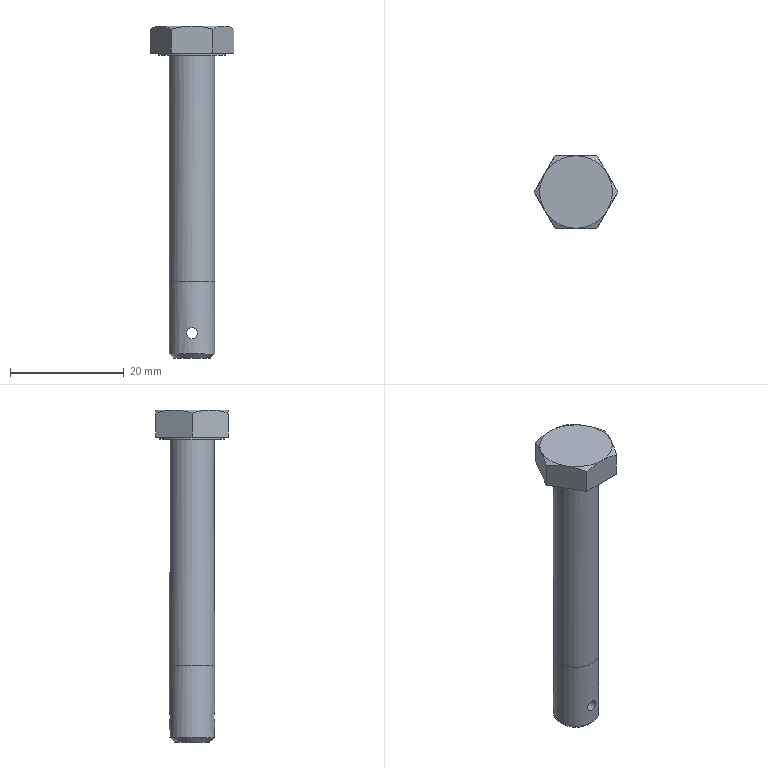Part | NX | features solid 2 | 1 solid | 21 faces | box 14.723 x 12.751 x 58.363 mm | volume 3315 mm3 | plane 10 | cone 7 | cylinder 4 | commonest cylinder face diameters 7.938 x2 1.93 x1 11.684 x1
STEP:
#1=CARTESIAN_POINT('',(0.,-3.969,-54.962));
#2=VERTEX_POINT('',#1);
#3=CARTESIAN_POINT('',(0.7571,-3.91,-54.753));
#4=CARTESIAN_POINT('',(-0.000144,-3.998,-55.067));
#5=CARTESIAN_POINT('',(-0.7565,-3.91,-54.753));
#6=CARTESIAN_POINT('',(-1.07,-3.819,-53.998));
#7=CARTESIAN_POINT('',(-0.7564,-3.91,-53.241));
#8=CARTESIAN_POINT('',(-0.0004429,-3.998,-52.928));
#9=CARTESIAN_POINT('',(0.7557,-3.91,-53.24));
#10=CARTESIAN_POINT('',(1.07,-3.819,-53.997));
#11=CARTESIAN_POINT('',(0.7571,-3.91,-54.753));
#12=CARTESIAN_POINT('',(-0.000144,-3.998,-55.067));
#13=CARTESIAN_POINT('',(-0.7565,-3.91,-54.753));
#14=B_SPLINE_CURVE_WITH_KNOTS('',3,(#3,#4,#5,#6,#7,#8,#9,#10,#11,#12,#13),.UNSPECIFIED.,.T.,.F.,(1,1,1,1,1,1,1,1,1,1,1,1,1,1,1),(-0.002271,-0.001514,-0.0007572,0.,0.0007572,0.001514,0.002271,0.003029,0.003786,0.004543,0.0053,0.006057,0.006814,0.007572,0.008329),.UNSPECIFIED.);
#15=EDGE_CURVE('',#2,#2,#14,.T.);
#16=ORIENTED_EDGE('',*,*,#15,.T.);
#17=EDGE_LOOP('',(#16));
#18=FACE_BOUND('',#17,.T.);
#19=CARTESIAN_POINT('',(-3.969,0.,-44.869));
#20=VERTEX_POINT('',#19);
#21=CARTESIAN_POINT('',(-3.11,3.11,-44.869));
#22=CARTESIAN_POINT('',(-4.398,0.,-44.869));
#23=CARTESIAN_POINT('',(-3.11,-3.11,-44.869));
#24=CARTESIAN_POINT('',(0.,-4.398,-44.869));
#25=CARTESIAN_POINT('',(3.11,-3.11,-44.869));
#26=CARTESIAN_POINT('',(4.398,0.,-44.869));
#27=CARTESIAN_POINT('',(3.11,3.11,-44.869));
#28=CARTESIAN_POINT('',(0.,4.398,-44.869));
#29=CARTESIAN_POINT('',(-3.11,3.11,-44.869));
#30=CARTESIAN_POINT('',(-4.398,0.,-44.869));
#31=CARTESIAN_POINT('',(-3.11,-3.11,-44.869));
#32=B_SPLINE_CURVE_WITH_KNOTS('',3,(#21,#22,#23,#24,#25,#26,#27,#28,#29,#30,#31),.UNSPECIFIED.,.T.,.F.,(1,1,1,1,1,1,1,1,1,1,1,1,1,1,1),(-0.375,-0.25,-0.125,0.,0.125,0.25,0.375,0.5,0.625,0.75,0.875,1.,1.125,1.25,1.375),.UNSPECIFIED.);
#33=EDGE_CURVE('',#20,#20,#32,.T.);
#34=ORIENTED_EDGE('',*,*,#33,.F.);
#35=EDGE_LOOP('',(#34));
#36=FACE_BOUND('',#35,.T.);
#37=CARTESIAN_POINT('',(-3.969,0.,-57.575));
#38=VERTEX_POINT('',#37);
#39=CARTESIAN_POINT('',(0.,0.,-57.575));
#40=DIRECTION('',(0.,0.,-1.));
#41=DIRECTION('',(-1.,0.,0.));
#42=AXIS2_PLACEMENT_3D('',#39,#40,#41);
#43=CIRCLE('',#42,3.969);
#44=EDGE_CURVE('',#38,#38,#43,.T.);
#45=ORIENTED_EDGE('',*,*,#44,.F.);
#46=EDGE_LOOP('',(#45));
#47=FACE_BOUND('',#46,.T.);
#48=CARTESIAN_POINT('',(0.,3.969,-54.962));
#49=VERTEX_POINT('',#48);
#50=CARTESIAN_POINT('',(-0.7571,3.91,-54.753));
#51=CARTESIAN_POINT('',(0.000144,3.998,-55.067));
#52=CARTESIAN_POINT('',(0.7565,3.91,-54.753));
#53=CARTESIAN_POINT('',(1.07,3.819,-53.998));
#54=CARTESIAN_POINT('',(0.7564,3.91,-53.241));
#55=CARTESIAN_POINT('',(0.0004429,3.998,-52.928));
#56=CARTESIAN_POINT('',(-0.7557,3.91,-53.24));
#57=CARTESIAN_POINT('',(-1.07,3.819,-53.997));
#58=CARTESIAN_POINT('',(-0.7571,3.91,-54.753));
#59=CARTESIAN_POINT('',(0.000144,3.998,-55.067));
#60=CARTESIAN_POINT('',(0.7565,3.91,-54.753));
#61=B_SPLINE_CURVE_WITH_KNOTS('',3,(#50,#51,#52,#53,#54,#55,#56,#57,#58,#59,#60),.UNSPECIFIED.,.T.,.F.,(1,1,1,1,1,1,1,1,1,1,1,1,1,1,1),(-0.002271,-0.001514,-0.0007572,0.,0.0007572,0.001514,0.002271,0.003029,0.003786,0.004543,0.0053,0.006057,0.006814,0.007572,0.008329),.UNSPECIFIED.);
#62=EDGE_CURVE('',#49,#49,#61,.T.);
#63=ORIENTED_EDGE('',*,*,#62,.T.);
#64=EDGE_LOOP('',(#63));
#65=FACE_BOUND('',#64,.T.);
#66=CARTESIAN_POINT('',(0.,0.,0.));
#67=DIRECTION('',(0.,0.,-1.));
#68=DIRECTION('',(-1.,0.,0.));
#69=AXIS2_PLACEMENT_3D('',#66,#67,#68);
#70=CYLINDRICAL_SURFACE('',#69,3.969);
#71=ADVANCED_FACE('',(#18,#36,#47,#65),#70,.T.);
#72=CARTESIAN_POINT('',(-3.969,0.,-5.182));
#73=VERTEX_POINT('',#72);
#74=CARTESIAN_POINT('',(0.,0.,-5.182));
#75=DIRECTION('',(0.,0.,-1.));
#76=DIRECTION('',(-1.,0.,0.));
#77=AXIS2_PLACEMENT_3D('',#74,#75,#76);
#78=CIRCLE('',#77,3.969);
#79=EDGE_CURVE('',#73,#73,#78,.T.);
#80=ORIENTED_EDGE('',*,*,#79,.T.);
#81=EDGE_LOOP('',(#80));
#82=FACE_BOUND('',#81,.T.);
#83=ORIENTED_EDGE('',*,*,#33,.T.);
#84=EDGE_LOOP('',(#83));
#85=FACE_BOUND('',#84,.T.);
#86=CARTESIAN_POINT('',(0.,0.,0.));
#87=DIRECTION('',(0.,0.,-1.));
#88=DIRECTION('',(-1.,0.,0.));
#89=AXIS2_PLACEMENT_3D('',#86,#87,#88);
#90=CYLINDRICAL_SURFACE('',#89,3.969);
#91=ADVANCED_FACE('',(#82,#85),#90,.T.);
#92=CARTESIAN_POINT('',(-7.362,0.,-4.775));
#93=VERTEX_POINT('',#92);
#94=CARTESIAN_POINT('',(-3.681,6.375,-4.775));
#95=VERTEX_POINT('',#94);
#96=CARTESIAN_POINT('',(-4.061,5.717,-4.775));
#97=DIRECTION('',(0.5,0.866,0.));
#98=VECTOR('',#97,1000.);
#99=LINE('',#96,#98);
#100=EDGE_CURVE('',#93,#95,#99,.T.);
#101=ORIENTED_EDGE('',*,*,#100,.T.);
#102=CARTESIAN_POINT('',(3.681,6.375,-4.775));
#103=VERTEX_POINT('',#102);
#104=CARTESIAN_POINT('',(5.842,6.375,-4.775));
#105=DIRECTION('',(1.,0.,0.));
#106=VECTOR('',#105,1000.);
#107=LINE('',#104,#106);
#108=EDGE_CURVE('',#95,#103,#107,.T.);
#109=ORIENTED_EDGE('',*,*,#108,.T.);
#110=CARTESIAN_POINT('',(7.362,0.,-4.775));
#111=VERTEX_POINT('',#110);
#112=CARTESIAN_POINT('',(6.982,0.658,-4.775));
#113=DIRECTION('',(0.5,-0.866,0.));
#114=VECTOR('',#113,1000.);
#115=LINE('',#112,#114);
#116=EDGE_CURVE('',#103,#111,#115,.T.);
#117=ORIENTED_EDGE('',*,*,#116,.T.);
#118=CARTESIAN_POINT('',(3.681,-6.375,-4.775));
#119=VERTEX_POINT('',#118);
#120=CARTESIAN_POINT('',(6.982,-0.658,-4.775));
#121=DIRECTION('',(-0.5,-0.866,0.));
#122=VECTOR('',#121,1000.);
#123=LINE('',#120,#122);
#124=EDGE_CURVE('',#111,#119,#123,.T.);
#125=ORIENTED_EDGE('',*,*,#124,.T.);
#126=CARTESIAN_POINT('',(-3.681,-6.375,-4.775));
#127=VERTEX_POINT('',#126);
#128=CARTESIAN_POINT('',(5.842,-6.375,-4.775));
#129=DIRECTION('',(-1.,0.,0.));
#130=VECTOR('',#129,1000.);
#131=LINE('',#128,#130);
#132=EDGE_CURVE('',#119,#127,#131,.T.);
#133=ORIENTED_EDGE('',*,*,#132,.T.);
#134=CARTESIAN_POINT('',(-4.061,-5.717,-4.775));
#135=DIRECTION('',(-0.5,0.866,0.));
#136=VECTOR('',#135,1000.);
#137=LINE('',#134,#136);
#138=EDGE_CURVE('',#127,#93,#137,.T.);
#139=ORIENTED_EDGE('',*,*,#138,.T.);
#140=EDGE_LOOP('',(#101,#109,#117,#125,#133,#139));
#141=FACE_BOUND('',#140,.T.);
#142=CARTESIAN_POINT('',(-5.842,0.,-4.775));
#143=VERTEX_POINT('',#142);
#144=CARTESIAN_POINT('',(0.,0.,-4.775));
#145=DIRECTION('',(0.,0.,-1.));
#146=DIRECTION('',(-1.,0.,0.));
#147=AXIS2_PLACEMENT_3D('',#144,#145,#146);
#148=CIRCLE('',#147,5.842);
#149=EDGE_CURVE('',#143,#143,#148,.T.);
#150=ORIENTED_EDGE('',*,*,#149,.F.);
#151=EDGE_LOOP('',(#150));
#152=FACE_BOUND('',#151,.T.);
#153=CARTESIAN_POINT('',(5.842,0.,-4.775));
#154=DIRECTION('',(0.,0.,-1.));
#155=DIRECTION('',(-1.,0.,0.));
#156=AXIS2_PLACEMENT_3D('',#153,#154,#155);
#157=PLANE('',#156);
#158=ADVANCED_FACE('',(#141,#152),#157,.T.);
#159=CARTESIAN_POINT('',(-3.181,0.,-58.363));
#160=VERTEX_POINT('',#159);
#161=CARTESIAN_POINT('',(0.,0.,-58.363));
#162=DIRECTION('',(0.,0.,-1.));
#163=DIRECTION('',(-1.,0.,0.));
#164=AXIS2_PLACEMENT_3D('',#161,#162,#163);
#165=CIRCLE('',#164,3.181);
#166=EDGE_CURVE('',#160,#160,#165,.T.);
#167=ORIENTED_EDGE('',*,*,#166,.T.);
#168=EDGE_LOOP('',(#167));
#169=FACE_BOUND('',#168,.T.);
#170=CARTESIAN_POINT('',(0.,0.,-58.363));
#171=DIRECTION('',(0.,0.,-1.));
#172=DIRECTION('',(-1.,0.,0.));
#173=AXIS2_PLACEMENT_3D('',#170,#171,#172);
#174=PLANE('',#173);
#175=ADVANCED_FACE('',(#169),#174,.T.);
#176=ORIENTED_EDGE('',*,*,#44,.T.);
#177=EDGE_LOOP('',(#176));
#178=FACE_BOUND('',#177,.T.);
#179=ORIENTED_EDGE('',*,*,#166,.F.);
#180=EDGE_LOOP('',(#179));
#181=FACE_BOUND('',#180,.T.);
#182=CARTESIAN_POINT('',(0.,0.,-58.363));
#183=DIRECTION('',(0.,0.,1.));
#184=DIRECTION('',(1.,0.,0.));
#185=AXIS2_PLACEMENT_3D('',#182,#183,#184);
#186=CONICAL_SURFACE('',#185,3.181,0.7854);
#187=ADVANCED_FACE('',(#178,#181),#186,.T.);
#188=CARTESIAN_POINT('',(-5.842,0.,-5.182));
#189=VERTEX_POINT('',#188);
#190=CARTESIAN_POINT('',(0.,0.,-5.182));
#191=DIRECTION('',(0.,0.,-1.));
#192=DIRECTION('',(-1.,0.,0.));
#193=AXIS2_PLACEMENT_3D('',#190,#191,#192);
#194=CIRCLE('',#193,5.842);
#195=EDGE_CURVE('',#189,#189,#194,.T.);
#196=ORIENTED_EDGE('',*,*,#195,.T.);
#197=EDGE_LOOP('',(#196));
#198=FACE_BOUND('',#197,.T.);
#199=ORIENTED_EDGE('',*,*,#79,.F.);
#200=EDGE_LOOP('',(#199));
#201=FACE_BOUND('',#200,.T.);
#202=CARTESIAN_POINT('',(3.969,0.,-5.182));
#203=DIRECTION('',(0.,0.,-1.));
#204=DIRECTION('',(-1.,0.,0.));
#205=AXIS2_PLACEMENT_3D('',#202,#203,#204);
#206=PLANE('',#205);
#207=ADVANCED_FACE('',(#198,#201),#206,.T.);
#208=ORIENTED_EDGE('',*,*,#149,.T.);
#209=EDGE_LOOP('',(#208));
#210=FACE_BOUND('',#209,.T.);
#211=ORIENTED_EDGE('',*,*,#195,.F.);
#212=EDGE_LOOP('',(#211));
#213=FACE_BOUND('',#212,.T.);
#214=CARTESIAN_POINT('',(0.,0.,0.));
#215=DIRECTION('',(0.,0.,-1.));
#216=DIRECTION('',(-1.,0.,0.));
#217=AXIS2_PLACEMENT_3D('',#214,#215,#216);
#218=CYLINDRICAL_SURFACE('',#217,5.842);
#219=ADVANCED_FACE('',(#210,#213),#218,.T.);
#220=ORIENTED_EDGE('',*,*,#108,.F.);
#221=CARTESIAN_POINT('',(-3.681,6.375,-0.5694));
#222=VERTEX_POINT('',#221);
#223=CARTESIAN_POINT('',(-3.681,6.375,-64.199));
#224=DIRECTION('',(0.,0.,1.));
#225=VECTOR('',#224,1000.);
#226=LINE('',#223,#225);
#227=EDGE_CURVE('',#95,#222,#226,.T.);
#228=ORIENTED_EDGE('',*,*,#227,.T.);
#229=CARTESIAN_POINT('',(0.,6.375,0.));
#230=VERTEX_POINT('',#229);
#231=CARTESIAN_POINT('',(-3.681,6.375,-0.5694));
#232=CARTESIAN_POINT('',(-2.484,6.375,-0.2238));
#233=CARTESIAN_POINT('',(-1.244,6.375,0.));
#234=CARTESIAN_POINT('',(0.,6.375,0.));
#235=B_SPLINE_CURVE_WITH_KNOTS('',3,(#231,#232,#233,#234),.UNSPECIFIED.,.F.,.F.,(4,4),(0.006567,0.01029),.UNSPECIFIED.);
#236=EDGE_CURVE('',#230,#222,#235,.F.);
#237=ORIENTED_EDGE('',*,*,#236,.F.);
#238=CARTESIAN_POINT('',(3.681,6.375,-0.5694));
#239=VERTEX_POINT('',#238);
#240=CARTESIAN_POINT('',(0.,6.375,0.));
#241=CARTESIAN_POINT('',(1.245,6.375,0.));
#242=CARTESIAN_POINT('',(2.49,6.375,-0.2258));
#243=CARTESIAN_POINT('',(3.681,6.375,-0.5694));
#244=B_SPLINE_CURVE_WITH_KNOTS('',3,(#240,#241,#242,#243),.UNSPECIFIED.,.F.,.F.,(4,4),(0.01029,0.01402),.UNSPECIFIED.);
#245=EDGE_CURVE('',#239,#230,#244,.F.);
#246=ORIENTED_EDGE('',*,*,#245,.F.);
#247=CARTESIAN_POINT('',(3.681,6.375,-64.199));
#248=DIRECTION('',(0.,0.,1.));
#249=VECTOR('',#248,1000.);
#250=LINE('',#247,#249);
#251=EDGE_CURVE('',#103,#239,#250,.T.);
#252=ORIENTED_EDGE('',*,*,#251,.F.);
#253=EDGE_LOOP('',(#220,#228,#237,#246,#252));
#254=FACE_BOUND('',#253,.T.);
#255=CARTESIAN_POINT('',(3.681,6.375,-64.199));
#256=DIRECTION('',(0.,1.,0.));
#257=DIRECTION('',(0.,0.,1.));
#258=AXIS2_PLACEMENT_3D('',#255,#256,#257);
#259=PLANE('',#258);
#260=ADVANCED_FACE('',(#254),#259,.T.);
#261=ORIENTED_EDGE('',*,*,#100,.F.);
#262=CARTESIAN_POINT('',(-7.362,0.,-0.5694));
#263=VERTEX_POINT('',#262);
#264=CARTESIAN_POINT('',(-7.362,0.,-64.199));
#265=DIRECTION('',(0.,0.,1.));
#266=VECTOR('',#265,1000.);
#267=LINE('',#264,#266);
#268=EDGE_CURVE('',#93,#263,#267,.T.);
#269=ORIENTED_EDGE('',*,*,#268,.T.);
#270=CARTESIAN_POINT('',(-5.521,3.188,0.));
#271=VERTEX_POINT('',#270);
#272=CARTESIAN_POINT('',(-5.521,3.188,0.));
#273=CARTESIAN_POINT('',(-6.146,2.106,0.));
#274=CARTESIAN_POINT('',(-6.761,1.04,-0.2227));
#275=CARTESIAN_POINT('',(-7.362,0.,-0.5694));
#276=B_SPLINE_CURVE_WITH_KNOTS('',3,(#272,#273,#274,#275),.UNSPECIFIED.,.F.,.F.,(4,4),(0.003725,0.007435),.UNSPECIFIED.);
#277=EDGE_CURVE('',#271,#263,#276,.T.);
#278=ORIENTED_EDGE('',*,*,#277,.F.);
#279=CARTESIAN_POINT('',(-3.681,6.375,-0.5694));
#280=CARTESIAN_POINT('',(-4.283,5.332,-0.2218));
#281=CARTESIAN_POINT('',(-4.894,4.274,0.));
#282=CARTESIAN_POINT('',(-5.521,3.188,0.));
#283=B_SPLINE_CURVE_WITH_KNOTS('',3,(#279,#280,#281,#282),.UNSPECIFIED.,.F.,.F.,(4,4),(0.000000238,0.003725),.UNSPECIFIED.);
#284=EDGE_CURVE('',#222,#271,#283,.T.);
#285=ORIENTED_EDGE('',*,*,#284,.F.);
#286=ORIENTED_EDGE('',*,*,#227,.F.);
#287=EDGE_LOOP('',(#261,#269,#278,#285,#286));
#288=FACE_BOUND('',#287,.T.);
#289=CARTESIAN_POINT('',(-3.681,6.375,-64.199));
#290=DIRECTION('',(-0.866,0.5,0.));
#291=DIRECTION('',(-0.5,-0.866,0.));
#292=AXIS2_PLACEMENT_3D('',#289,#290,#291);
#293=PLANE('',#292);
#294=ADVANCED_FACE('',(#288),#293,.T.);
#295=ORIENTED_EDGE('',*,*,#138,.F.);
#296=CARTESIAN_POINT('',(-3.681,-6.375,-0.5694));
#297=VERTEX_POINT('',#296);
#298=CARTESIAN_POINT('',(-3.681,-6.375,-64.199));
#299=DIRECTION('',(0.,0.,1.));
#300=VECTOR('',#299,1000.);
#301=LINE('',#298,#300);
#302=EDGE_CURVE('',#127,#297,#301,.T.);
#303=ORIENTED_EDGE('',*,*,#302,.T.);
#304=CARTESIAN_POINT('',(-5.521,-3.188,0.));
#305=VERTEX_POINT('',#304);
#306=CARTESIAN_POINT('',(-5.521,-3.188,0.));
#307=CARTESIAN_POINT('',(-4.896,-4.27,0.));
#308=CARTESIAN_POINT('',(-4.281,-5.335,-0.2227));
#309=CARTESIAN_POINT('',(-3.681,-6.375,-0.5694));
#310=B_SPLINE_CURVE_WITH_KNOTS('',3,(#306,#307,#308,#309),.UNSPECIFIED.,.F.,.F.,(4,4),(0.003725,0.007435),.UNSPECIFIED.);
#311=EDGE_CURVE('',#305,#297,#310,.T.);
#312=ORIENTED_EDGE('',*,*,#311,.F.);
#313=CARTESIAN_POINT('',(-7.362,0.,-0.5694));
#314=CARTESIAN_POINT('',(-6.76,-1.043,-0.2218));
#315=CARTESIAN_POINT('',(-6.148,-2.102,0.));
#316=CARTESIAN_POINT('',(-5.521,-3.188,0.));
#317=B_SPLINE_CURVE_WITH_KNOTS('',3,(#313,#314,#315,#316),.UNSPECIFIED.,.F.,.F.,(4,4),(0.000000238,0.003725),.UNSPECIFIED.);
#318=EDGE_CURVE('',#263,#305,#317,.T.);
#319=ORIENTED_EDGE('',*,*,#318,.F.);
#320=ORIENTED_EDGE('',*,*,#268,.F.);
#321=EDGE_LOOP('',(#295,#303,#312,#319,#320));
#322=FACE_BOUND('',#321,.T.);
#323=CARTESIAN_POINT('',(-7.362,0.,-64.199));
#324=DIRECTION('',(-0.866,-0.5,0.));
#325=DIRECTION('',(0.5,-0.866,0.));
#326=AXIS2_PLACEMENT_3D('',#323,#324,#325);
#327=PLANE('',#326);
#328=ADVANCED_FACE('',(#322),#327,.T.);
#329=ORIENTED_EDGE('',*,*,#132,.F.);
#330=CARTESIAN_POINT('',(3.681,-6.375,-0.5694));
#331=VERTEX_POINT('',#330);
#332=CARTESIAN_POINT('',(3.681,-6.375,-64.199));
#333=DIRECTION('',(0.,0.,1.));
#334=VECTOR('',#333,1000.);
#335=LINE('',#332,#334);
#336=EDGE_CURVE('',#119,#331,#335,.T.);
#337=ORIENTED_EDGE('',*,*,#336,.T.);
#338=CARTESIAN_POINT('',(0.,-6.375,0.));
#339=VERTEX_POINT('',#338);
#340=CARTESIAN_POINT('',(0.,-6.375,0.));
#341=CARTESIAN_POINT('',(1.245,-6.375,0.));
#342=CARTESIAN_POINT('',(2.49,-6.375,-0.2258));
#343=CARTESIAN_POINT('',(3.681,-6.375,-0.5694));
#344=B_SPLINE_CURVE_WITH_KNOTS('',3,(#340,#341,#342,#343),.UNSPECIFIED.,.F.,.F.,(4,4),(0.01029,0.01402),.UNSPECIFIED.);
#345=EDGE_CURVE('',#339,#331,#344,.T.);
#346=ORIENTED_EDGE('',*,*,#345,.F.);
#347=CARTESIAN_POINT('',(-3.681,-6.375,-0.5694));
#348=CARTESIAN_POINT('',(-2.484,-6.375,-0.2238));
#349=CARTESIAN_POINT('',(-1.244,-6.375,0.));
#350=CARTESIAN_POINT('',(0.,-6.375,0.));
#351=B_SPLINE_CURVE_WITH_KNOTS('',3,(#347,#348,#349,#350),.UNSPECIFIED.,.F.,.F.,(4,4),(0.006567,0.01029),.UNSPECIFIED.);
#352=EDGE_CURVE('',#297,#339,#351,.T.);
#353=ORIENTED_EDGE('',*,*,#352,.F.);
#354=ORIENTED_EDGE('',*,*,#302,.F.);
#355=EDGE_LOOP('',(#329,#337,#346,#353,#354));
#356=FACE_BOUND('',#355,.T.);
#357=CARTESIAN_POINT('',(-3.681,-6.375,-64.199));
#358=DIRECTION('',(0.,-1.,0.));
#359=DIRECTION('',(0.,0.,-1.));
#360=AXIS2_PLACEMENT_3D('',#357,#358,#359);
#361=PLANE('',#360);
#362=ADVANCED_FACE('',(#356),#361,.T.);
#363=ORIENTED_EDGE('',*,*,#124,.F.);
#364=CARTESIAN_POINT('',(7.362,0.,-0.5694));
#365=VERTEX_POINT('',#364);
#366=CARTESIAN_POINT('',(7.362,0.,-64.199));
#367=DIRECTION('',(0.,0.,1.));
#368=VECTOR('',#367,1000.);
#369=LINE('',#366,#368);
#370=EDGE_CURVE('',#111,#365,#369,.T.);
#371=ORIENTED_EDGE('',*,*,#370,.T.);
#372=CARTESIAN_POINT('',(5.521,-3.188,0.));
#373=VERTEX_POINT('',#372);
#374=CARTESIAN_POINT('',(5.521,-3.188,0.));
#375=CARTESIAN_POINT('',(6.146,-2.106,0.));
#376=CARTESIAN_POINT('',(6.761,-1.04,-0.2227));
#377=CARTESIAN_POINT('',(7.362,0.,-0.5694));
#378=B_SPLINE_CURVE_WITH_KNOTS('',3,(#374,#375,#376,#377),.UNSPECIFIED.,.F.,.F.,(4,4),(0.003725,0.007435),.UNSPECIFIED.);
#379=EDGE_CURVE('',#373,#365,#378,.T.);
#380=ORIENTED_EDGE('',*,*,#379,.F.);
#381=CARTESIAN_POINT('',(3.681,-6.375,-0.5694));
#382=CARTESIAN_POINT('',(4.283,-5.332,-0.2218));
#383=CARTESIAN_POINT('',(4.894,-4.274,0.));
#384=CARTESIAN_POINT('',(5.521,-3.188,0.));
#385=B_SPLINE_CURVE_WITH_KNOTS('',3,(#381,#382,#383,#384),.UNSPECIFIED.,.F.,.F.,(4,4),(0.000000238,0.003725),.UNSPECIFIED.);
#386=EDGE_CURVE('',#331,#373,#385,.T.);
#387=ORIENTED_EDGE('',*,*,#386,.F.);
#388=ORIENTED_EDGE('',*,*,#336,.F.);
#389=EDGE_LOOP('',(#363,#371,#380,#387,#388));
#390=FACE_BOUND('',#389,.T.);
#391=CARTESIAN_POINT('',(3.681,-6.375,-64.199));
#392=DIRECTION('',(0.866,-0.5,0.));
#393=DIRECTION('',(0.5,0.866,0.));
#394=AXIS2_PLACEMENT_3D('',#391,#392,#393);
#395=PLANE('',#394);
#396=ADVANCED_FACE('',(#390),#395,.T.);
#397=ORIENTED_EDGE('',*,*,#116,.F.);
#398=ORIENTED_EDGE('',*,*,#251,.T.);
#399=CARTESIAN_POINT('',(5.521,3.188,0.));
#400=VERTEX_POINT('',#399);
#401=CARTESIAN_POINT('',(5.521,3.188,0.));
#402=CARTESIAN_POINT('',(4.896,4.27,0.));
#403=CARTESIAN_POINT('',(4.281,5.335,-0.2227));
#404=CARTESIAN_POINT('',(3.681,6.375,-0.5694));
#405=B_SPLINE_CURVE_WITH_KNOTS('',3,(#401,#402,#403,#404),.UNSPECIFIED.,.F.,.F.,(4,4),(0.003725,0.007435),.UNSPECIFIED.);
#406=EDGE_CURVE('',#400,#239,#405,.T.);
#407=ORIENTED_EDGE('',*,*,#406,.F.);
#408=CARTESIAN_POINT('',(7.362,0.,-0.5694));
#409=CARTESIAN_POINT('',(6.76,1.043,-0.2218));
#410=CARTESIAN_POINT('',(6.148,2.102,0.));
#411=CARTESIAN_POINT('',(5.521,3.188,0.));
#412=B_SPLINE_CURVE_WITH_KNOTS('',3,(#408,#409,#410,#411),.UNSPECIFIED.,.F.,.F.,(4,4),(0.000000238,0.003725),.UNSPECIFIED.);
#413=EDGE_CURVE('',#365,#400,#412,.T.);
#414=ORIENTED_EDGE('',*,*,#413,.F.);
#415=ORIENTED_EDGE('',*,*,#370,.F.);
#416=EDGE_LOOP('',(#397,#398,#407,#414,#415));
#417=FACE_BOUND('',#416,.T.);
#418=CARTESIAN_POINT('',(7.362,0.,-64.199));
#419=DIRECTION('',(0.866,0.5,0.));
#420=DIRECTION('',(-0.5,0.866,0.));
#421=AXIS2_PLACEMENT_3D('',#418,#419,#420);
#422=PLANE('',#421);
#423=ADVANCED_FACE('',(#417),#422,.T.);
#424=CARTESIAN_POINT('',(0.,0.,0.));
#425=DIRECTION('',(0.,0.,-1.));
#426=DIRECTION('',(-1.,0.,0.));
#427=AXIS2_PLACEMENT_3D('',#424,#425,#426);
#428=CIRCLE('',#427,6.375);
#429=EDGE_CURVE('',#400,#373,#428,.T.);
#430=ORIENTED_EDGE('',*,*,#429,.T.);
#431=ORIENTED_EDGE('',*,*,#379,.T.);
#432=ORIENTED_EDGE('',*,*,#413,.T.);
#433=EDGE_LOOP('',(#430,#431,#432));
#434=FACE_BOUND('',#433,.T.);
#435=CARTESIAN_POINT('',(0.,0.,-0.5719));
#436=DIRECTION('',(0.,0.,-1.));
#437=DIRECTION('',(-1.,0.,0.));
#438=AXIS2_PLACEMENT_3D('',#435,#436,#437);
#439=CONICAL_SURFACE('',#438,7.366,1.047);
#440=ADVANCED_FACE('',(#434),#439,.T.);
#441=CARTESIAN_POINT('',(0.,0.,0.));
#442=DIRECTION('',(0.,0.,-1.));
#443=DIRECTION('',(-1.,0.,0.));
#444=AXIS2_PLACEMENT_3D('',#441,#442,#443);
#445=CIRCLE('',#444,6.375);
#446=EDGE_CURVE('',#373,#339,#445,.T.);
#447=ORIENTED_EDGE('',*,*,#446,.T.);
#448=ORIENTED_EDGE('',*,*,#345,.T.);
#449=ORIENTED_EDGE('',*,*,#386,.T.);
#450=EDGE_LOOP('',(#447,#448,#449));
#451=FACE_BOUND('',#450,.T.);
#452=CARTESIAN_POINT('',(0.,0.,-0.5719));
#453=DIRECTION('',(0.,0.,-1.));
#454=DIRECTION('',(-1.,0.,0.));
#455=AXIS2_PLACEMENT_3D('',#452,#453,#454);
#456=CONICAL_SURFACE('',#455,7.366,1.047);
#457=ADVANCED_FACE('',(#451),#456,.T.);
#458=CARTESIAN_POINT('',(0.,0.,0.));
#459=DIRECTION('',(0.,0.,-1.));
#460=DIRECTION('',(-1.,0.,0.));
#461=AXIS2_PLACEMENT_3D('',#458,#459,#460);
#462=CIRCLE('',#461,6.375);
#463=EDGE_CURVE('',#339,#305,#462,.T.);
#464=ORIENTED_EDGE('',*,*,#463,.T.);
#465=ORIENTED_EDGE('',*,*,#311,.T.);
#466=ORIENTED_EDGE('',*,*,#352,.T.);
#467=EDGE_LOOP('',(#464,#465,#466));
#468=FACE_BOUND('',#467,.T.);
#469=CARTESIAN_POINT('',(0.,0.,-0.5719));
#470=DIRECTION('',(0.,0.,-1.));
#471=DIRECTION('',(-1.,0.,0.));
#472=AXIS2_PLACEMENT_3D('',#469,#470,#471);
#473=CONICAL_SURFACE('',#472,7.366,1.047);
#474=ADVANCED_FACE('',(#468),#473,.T.);
#475=CARTESIAN_POINT('',(0.,0.,0.));
#476=DIRECTION('',(0.,0.,-1.));
#477=DIRECTION('',(-1.,0.,0.));
#478=AXIS2_PLACEMENT_3D('',#475,#476,#477);
#479=CIRCLE('',#478,6.375);
#480=EDGE_CURVE('',#305,#271,#479,.T.);
#481=ORIENTED_EDGE('',*,*,#480,.T.);
#482=ORIENTED_EDGE('',*,*,#277,.T.);
#483=ORIENTED_EDGE('',*,*,#318,.T.);
#484=EDGE_LOOP('',(#481,#482,#483));
#485=FACE_BOUND('',#484,.T.);
#486=CARTESIAN_POINT('',(0.,0.,-0.5719));
#487=DIRECTION('',(0.,0.,-1.));
#488=DIRECTION('',(-1.,0.,0.));
#489=AXIS2_PLACEMENT_3D('',#486,#487,#488);
#490=CONICAL_SURFACE('',#489,7.366,1.047);
#491=ADVANCED_FACE('',(#485),#490,.T.);
#492=CARTESIAN_POINT('',(0.,0.,0.));
#493=DIRECTION('',(0.,0.,-1.));
#494=DIRECTION('',(-1.,0.,0.));
#495=AXIS2_PLACEMENT_3D('',#492,#493,#494);
#496=CIRCLE('',#495,6.375);
#497=EDGE_CURVE('',#271,#230,#496,.T.);
#498=ORIENTED_EDGE('',*,*,#497,.T.);
#499=ORIENTED_EDGE('',*,*,#236,.T.);
#500=ORIENTED_EDGE('',*,*,#284,.T.);
#501=EDGE_LOOP('',(#498,#499,#500));
#502=FACE_BOUND('',#501,.T.);
#503=CARTESIAN_POINT('',(0.,0.,-0.5719));
#504=DIRECTION('',(0.,0.,-1.));
#505=DIRECTION('',(-1.,0.,0.));
#506=AXIS2_PLACEMENT_3D('',#503,#504,#505);
#507=CONICAL_SURFACE('',#506,7.366,1.047);
#508=ADVANCED_FACE('',(#502),#507,.T.);
#509=ORIENTED_EDGE('',*,*,#497,.F.);
#510=ORIENTED_EDGE('',*,*,#480,.F.);
#511=ORIENTED_EDGE('',*,*,#463,.F.);
#512=ORIENTED_EDGE('',*,*,#446,.F.);
#513=ORIENTED_EDGE('',*,*,#429,.F.);
#514=CARTESIAN_POINT('',(0.,0.,0.));
#515=DIRECTION('',(0.,0.,-1.));
#516=DIRECTION('',(-1.,0.,0.));
#517=AXIS2_PLACEMENT_3D('',#514,#515,#516);
#518=CIRCLE('',#517,6.375);
#519=EDGE_CURVE('',#230,#400,#518,.T.);
#520=ORIENTED_EDGE('',*,*,#519,.F.);
#521=EDGE_LOOP('',(#509,#510,#511,#512,#513,#520));
#522=FACE_BOUND('',#521,.T.);
#523=CARTESIAN_POINT('',(6.375,0.,0.));
#524=DIRECTION('',(0.,0.,1.));
#525=DIRECTION('',(1.,0.,0.));
#526=AXIS2_PLACEMENT_3D('',#523,#524,#525);
#527=PLANE('',#526);
#528=ADVANCED_FACE('',(#522),#527,.T.);
#529=ORIENTED_EDGE('',*,*,#406,.T.);
#530=ORIENTED_EDGE('',*,*,#245,.T.);
#531=ORIENTED_EDGE('',*,*,#519,.T.);
#532=EDGE_LOOP('',(#529,#530,#531));
#533=FACE_BOUND('',#532,.T.);
#534=CARTESIAN_POINT('',(0.,0.,-0.5719));
#535=DIRECTION('',(0.,0.,-1.));
#536=DIRECTION('',(-1.,0.,0.));
#537=AXIS2_PLACEMENT_3D('',#534,#535,#536);
#538=CONICAL_SURFACE('',#537,7.366,1.047);
#539=ADVANCED_FACE('',(#533),#538,.T.);
#540=ORIENTED_EDGE('',*,*,#62,.F.);
#541=EDGE_LOOP('',(#540));
#542=FACE_BOUND('',#541,.T.);
#543=ORIENTED_EDGE('',*,*,#15,.F.);
#544=EDGE_LOOP('',(#543));
#545=FACE_BOUND('',#544,.T.);
#546=CARTESIAN_POINT('',(0.,7.013,-53.997));
#547=DIRECTION('',(0.,-1.,0.));
#548=DIRECTION('',(0.,0.,-1.));
#549=AXIS2_PLACEMENT_3D('',#546,#547,#548);
#550=CYLINDRICAL_SURFACE('',#549,0.9652);
#551=ADVANCED_FACE('',(#542,#545),#550,.F.);
#552=CLOSED_SHELL('',(#71,#91,#158,#175,#187,#207,#219,#260,#294,#328,#362,#396,#423,#440,#457,#474,#491,#508,#528,#539,#551));
#553=MANIFOLD_SOLID_BREP('',#552);
#554=(LENGTH_UNIT()NAMED_UNIT(*)SI_UNIT(.MILLI.,.METRE.));
#555=UNCERTAINTY_MEASURE_WITH_UNIT(LENGTH_MEASURE(0.0508),#554,'','');
#556=(NAMED_UNIT(*)PLANE_ANGLE_UNIT()SI_UNIT($,.RADIAN.));
#557=(NAMED_UNIT(*)SI_UNIT($,.STERADIAN.)SOLID_ANGLE_UNIT());
#558=(GEOMETRIC_REPRESENTATION_CONTEXT(3)GLOBAL_UNCERTAINTY_ASSIGNED_CONTEXT((#555))GLOBAL_UNIT_ASSIGNED_CONTEXT((#554,#556,#557))REPRESENTATION_CONTEXT('',''));
#559=ADVANCED_BREP_SHAPE_REPRESENTATION('',(#553),#558);